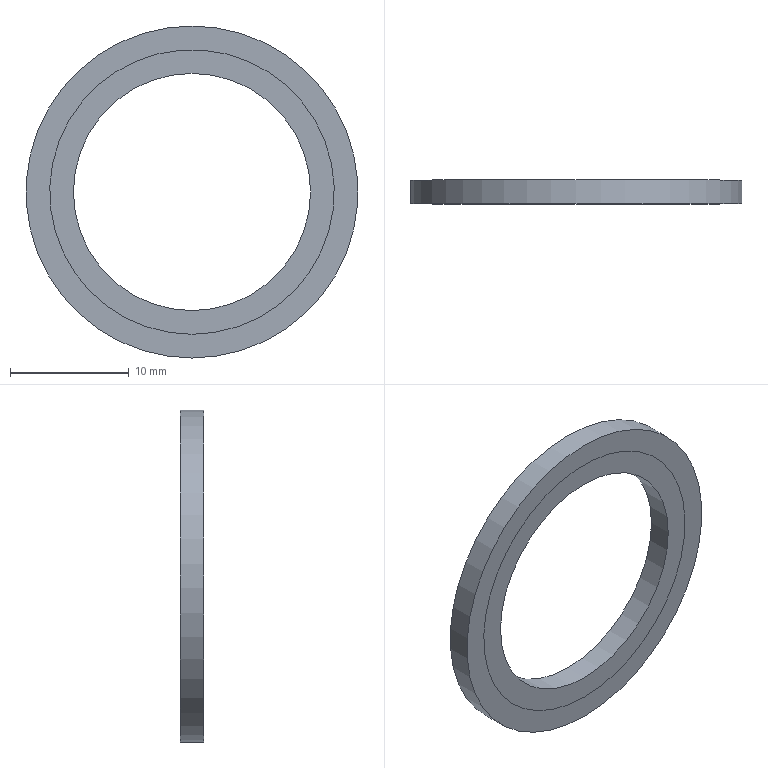Part | STEP file | 8903-ZTZD20 combined gasket | 2 solids | 8 faces | box 28 x 2 x 28 mm | volume 603.186 mm3 | plane 4 | cylinder 4 | commonest cylinder face diameters 24 x2 20 x1 28 x1
STEP:
#1=CARTESIAN_POINT('',(0.,0.,0.));
#2=DIRECTION('',(0.,0.,1.));
#3=DIRECTION('',(1.,0.,0.));
#4=AXIS2_PLACEMENT_3D('',#1,#2,#3);
#5=CARTESIAN_POINT('',(0.,2.,12.));
#6=VERTEX_POINT('',#5);
#7=CARTESIAN_POINT('',(0.,2.,-12.));
#8=VERTEX_POINT('',#7);
#9=CARTESIAN_POINT('',(0.,2.,0.));
#10=DIRECTION('',(0.,1.,0.));
#11=DIRECTION('',(0.,0.,1.));
#12=AXIS2_PLACEMENT_3D('',#9,#10,#11);
#13=CIRCLE('',#12,12.);
#14=CARTESIAN_POINT('',(0.,2.,0.));
#15=DIRECTION('',(0.,1.,0.));
#16=DIRECTION('',(0.,0.,1.));
#17=AXIS2_PLACEMENT_3D('',#14,#15,#16);
#18=PLANE('',#17);
#19=CARTESIAN_POINT('',(0.,0.));
#20=DIRECTION('',(1.,0.));
#21=AXIS2_PLACEMENT_2D('',#19,#20);
#22=CIRCLE('',#21,12.);
#23=(GEOMETRIC_REPRESENTATION_CONTEXT(2)PARAMETRIC_REPRESENTATION_CONTEXT()REPRESENTATION_CONTEXT('',''));
#24=DEFINITIONAL_REPRESENTATION('',(#22),#23);
#25=PCURVE('',#18,#24);
#26=CARTESIAN_POINT('',(0.,-38.212,0.));
#27=DIRECTION('',(0.,-1.,0.));
#28=DIRECTION('',(-1.,0.,0.));
#29=AXIS2_PLACEMENT_3D('',#26,#27,#28);
#30=CYLINDRICAL_SURFACE('',#29,12.);
#31=CARTESIAN_POINT('',(4.712,-40.212));
#32=DIRECTION('',(-1.,0.));
#33=VECTOR('',#32,1.);
#34=LINE('',#31,#33);
#35=(GEOMETRIC_REPRESENTATION_CONTEXT(2)PARAMETRIC_REPRESENTATION_CONTEXT()REPRESENTATION_CONTEXT('',''));
#36=DEFINITIONAL_REPRESENTATION('',(#34),#35);
#37=PCURVE('',#30,#36);
#38=SURFACE_CURVE('',#13,(#25,#37),.PCURVE_S1.);
#39=EDGE_CURVE('',#6,#8,#38,.T.);
#40=ORIENTED_EDGE('',*,*,#39,.F.);
#41=CARTESIAN_POINT('',(0.,2.,0.));
#42=DIRECTION('',(0.,1.,0.));
#43=DIRECTION('',(0.,0.,1.));
#44=AXIS2_PLACEMENT_3D('',#41,#42,#43);
#45=CIRCLE('',#44,12.);
#46=CARTESIAN_POINT('',(0.,0.));
#47=DIRECTION('',(1.,0.));
#48=AXIS2_PLACEMENT_2D('',#46,#47);
#49=CIRCLE('',#48,12.);
#50=(GEOMETRIC_REPRESENTATION_CONTEXT(2)PARAMETRIC_REPRESENTATION_CONTEXT()REPRESENTATION_CONTEXT('',''));
#51=DEFINITIONAL_REPRESENTATION('',(#49),#50);
#52=PCURVE('',#18,#51);
#53=CARTESIAN_POINT('',(10.996,-40.212));
#54=DIRECTION('',(-1.,0.));
#55=VECTOR('',#54,1.);
#56=LINE('',#53,#55);
#57=(GEOMETRIC_REPRESENTATION_CONTEXT(2)PARAMETRIC_REPRESENTATION_CONTEXT()REPRESENTATION_CONTEXT('',''));
#58=DEFINITIONAL_REPRESENTATION('',(#56),#57);
#59=PCURVE('',#30,#58);
#60=SURFACE_CURVE('',#45,(#52,#59),.PCURVE_S1.);
#61=EDGE_CURVE('',#8,#6,#60,.T.);
#62=ORIENTED_EDGE('',*,*,#61,.F.);
#63=EDGE_LOOP('',(#40,#62));
#64=FACE_BOUND('',#63,.T.);
#65=CARTESIAN_POINT('',(0.,2.,14.));
#66=VERTEX_POINT('',#65);
#67=CARTESIAN_POINT('',(0.,2.,-14.));
#68=VERTEX_POINT('',#67);
#69=CARTESIAN_POINT('',(0.,2.,0.));
#70=DIRECTION('',(0.,1.,0.));
#71=DIRECTION('',(0.,0.,1.));
#72=AXIS2_PLACEMENT_3D('',#69,#70,#71);
#73=CIRCLE('',#72,14.);
#74=CARTESIAN_POINT('',(0.,0.));
#75=DIRECTION('',(1.,0.));
#76=AXIS2_PLACEMENT_2D('',#74,#75);
#77=CIRCLE('',#76,14.);
#78=(GEOMETRIC_REPRESENTATION_CONTEXT(2)PARAMETRIC_REPRESENTATION_CONTEXT()REPRESENTATION_CONTEXT('',''));
#79=DEFINITIONAL_REPRESENTATION('',(#77),#78);
#80=PCURVE('',#18,#79);
#81=CARTESIAN_POINT('',(0.,-38.212,0.));
#82=DIRECTION('',(0.,-1.,0.));
#83=DIRECTION('',(-1.,0.,0.));
#84=AXIS2_PLACEMENT_3D('',#81,#82,#83);
#85=CYLINDRICAL_SURFACE('',#84,14.);
#86=CARTESIAN_POINT('',(4.712,-40.212));
#87=DIRECTION('',(-1.,0.));
#88=VECTOR('',#87,1.);
#89=LINE('',#86,#88);
#90=(GEOMETRIC_REPRESENTATION_CONTEXT(2)PARAMETRIC_REPRESENTATION_CONTEXT()REPRESENTATION_CONTEXT('',''));
#91=DEFINITIONAL_REPRESENTATION('',(#89),#90);
#92=PCURVE('',#85,#91);
#93=SURFACE_CURVE('',#73,(#80,#92),.PCURVE_S1.);
#94=EDGE_CURVE('',#66,#68,#93,.T.);
#95=ORIENTED_EDGE('',*,*,#94,.T.);
#96=CARTESIAN_POINT('',(0.,2.,0.));
#97=DIRECTION('',(0.,1.,0.));
#98=DIRECTION('',(0.,0.,1.));
#99=AXIS2_PLACEMENT_3D('',#96,#97,#98);
#100=CIRCLE('',#99,14.);
#101=CARTESIAN_POINT('',(0.,0.));
#102=DIRECTION('',(1.,0.));
#103=AXIS2_PLACEMENT_2D('',#101,#102);
#104=CIRCLE('',#103,14.);
#105=(GEOMETRIC_REPRESENTATION_CONTEXT(2)PARAMETRIC_REPRESENTATION_CONTEXT()REPRESENTATION_CONTEXT('',''));
#106=DEFINITIONAL_REPRESENTATION('',(#104),#105);
#107=PCURVE('',#18,#106);
#108=CARTESIAN_POINT('',(10.996,-40.212));
#109=DIRECTION('',(-1.,0.));
#110=VECTOR('',#109,1.);
#111=LINE('',#108,#110);
#112=(GEOMETRIC_REPRESENTATION_CONTEXT(2)PARAMETRIC_REPRESENTATION_CONTEXT()REPRESENTATION_CONTEXT('',''));
#113=DEFINITIONAL_REPRESENTATION('',(#111),#112);
#114=PCURVE('',#85,#113);
#115=SURFACE_CURVE('',#100,(#107,#114),.PCURVE_S1.);
#116=EDGE_CURVE('',#68,#66,#115,.T.);
#117=ORIENTED_EDGE('',*,*,#116,.T.);
#118=EDGE_LOOP('',(#95,#117));
#119=FACE_BOUND('',#118,.T.);
#120=ADVANCED_FACE('',(#64,#119),#18,.T.);
#121=CARTESIAN_POINT('',(0.,0.,-12.));
#122=VERTEX_POINT('',#121);
#123=CARTESIAN_POINT('',(0.,0.,0.));
#124=DIRECTION('',(0.,-1.,0.));
#125=DIRECTION('',(0.,0.,-1.));
#126=AXIS2_PLACEMENT_3D('',#123,#124,#125);
#127=CIRCLE('',#126,12.);
#128=CARTESIAN_POINT('',(0.,0.,0.));
#129=DIRECTION('',(0.,1.,0.));
#130=DIRECTION('',(0.,0.,1.));
#131=AXIS2_PLACEMENT_3D('',#128,#129,#130);
#132=PLANE('',#131);
#133=CARTESIAN_POINT('',(-12.,0.));
#134=CARTESIAN_POINT('',(-12.,20.785));
#135=CARTESIAN_POINT('',(6.,10.392));
#136=CARTESIAN_POINT('',(24.,0.));
#137=CARTESIAN_POINT('',(6.,-10.392));
#138=CARTESIAN_POINT('',(-12.,-20.785));
#139=CARTESIAN_POINT('',(-12.,0.));
#140=(BOUNDED_CURVE()B_SPLINE_CURVE(2,(#133,#134,#135,#136,#137,#138,#139),.UNSPECIFIED.,.T.,.F.)B_SPLINE_CURVE_WITH_KNOTS((1,2,2,2,2,1),(-2.094,0.,2.094,4.189,6.283,8.378),.UNSPECIFIED.)CURVE()GEOMETRIC_REPRESENTATION_ITEM()RATIONAL_B_SPLINE_CURVE((1.,0.5,1.,0.5,1.,0.5,1.))REPRESENTATION_ITEM(''));
#141=(GEOMETRIC_REPRESENTATION_CONTEXT(2)PARAMETRIC_REPRESENTATION_CONTEXT()REPRESENTATION_CONTEXT('',''));
#142=DEFINITIONAL_REPRESENTATION('',(#140),#141);
#143=PCURVE('',#132,#142);
#144=CARTESIAN_POINT('',(1.571,-38.212));
#145=DIRECTION('',(1.,0.));
#146=VECTOR('',#145,1.);
#147=LINE('',#144,#146);
#148=(GEOMETRIC_REPRESENTATION_CONTEXT(2)PARAMETRIC_REPRESENTATION_CONTEXT()REPRESENTATION_CONTEXT('',''));
#149=DEFINITIONAL_REPRESENTATION('',(#147),#148);
#150=PCURVE('',#30,#149);
#151=SURFACE_CURVE('',#127,(#143,#150),.PCURVE_S1.);
#152=EDGE_CURVE('',#122,#122,#151,.T.);
#153=ORIENTED_EDGE('',*,*,#152,.F.);
#154=EDGE_LOOP('',(#153));
#155=FACE_BOUND('',#154,.T.);
#156=CARTESIAN_POINT('',(0.,0.,-14.));
#157=VERTEX_POINT('',#156);
#158=CARTESIAN_POINT('',(0.,0.,0.));
#159=DIRECTION('',(0.,-1.,0.));
#160=DIRECTION('',(0.,0.,-1.));
#161=AXIS2_PLACEMENT_3D('',#158,#159,#160);
#162=CIRCLE('',#161,14.);
#163=CARTESIAN_POINT('',(-14.,0.));
#164=CARTESIAN_POINT('',(-14.,24.249));
#165=CARTESIAN_POINT('',(7.,12.124));
#166=CARTESIAN_POINT('',(28.,0.));
#167=CARTESIAN_POINT('',(7.,-12.124));
#168=CARTESIAN_POINT('',(-14.,-24.249));
#169=CARTESIAN_POINT('',(-14.,0.));
#170=(BOUNDED_CURVE()B_SPLINE_CURVE(2,(#163,#164,#165,#166,#167,#168,#169),.UNSPECIFIED.,.T.,.F.)B_SPLINE_CURVE_WITH_KNOTS((1,2,2,2,2,1),(-2.094,0.,2.094,4.189,6.283,8.378),.UNSPECIFIED.)CURVE()GEOMETRIC_REPRESENTATION_ITEM()RATIONAL_B_SPLINE_CURVE((1.,0.5,1.,0.5,1.,0.5,1.))REPRESENTATION_ITEM(''));
#171=(GEOMETRIC_REPRESENTATION_CONTEXT(2)PARAMETRIC_REPRESENTATION_CONTEXT()REPRESENTATION_CONTEXT('',''));
#172=DEFINITIONAL_REPRESENTATION('',(#170),#171);
#173=PCURVE('',#132,#172);
#174=CARTESIAN_POINT('',(1.571,-38.212));
#175=DIRECTION('',(1.,0.));
#176=VECTOR('',#175,1.);
#177=LINE('',#174,#176);
#178=(GEOMETRIC_REPRESENTATION_CONTEXT(2)PARAMETRIC_REPRESENTATION_CONTEXT()REPRESENTATION_CONTEXT('',''));
#179=DEFINITIONAL_REPRESENTATION('',(#177),#178);
#180=PCURVE('',#85,#179);
#181=SURFACE_CURVE('',#162,(#173,#180),.PCURVE_S1.);
#182=EDGE_CURVE('',#157,#157,#181,.T.);
#183=ORIENTED_EDGE('',*,*,#182,.T.);
#184=EDGE_LOOP('',(#183));
#185=FACE_BOUND('',#184,.T.);
#186=ADVANCED_FACE('',(#155,#185),#132,.F.);
#187=ORIENTED_EDGE('',*,*,#61,.F.);
#188=CARTESIAN_POINT('',(0.,2.,-12.));
#189=CARTESIAN_POINT('',(0.,0.,-12.));
#190=B_SPLINE_CURVE_WITH_KNOTS('',1,(#188,#189),.UNSPECIFIED.,.F.,.F.,(2,2),(-40.212,-38.212),.PIECEWISE_BEZIER_KNOTS.);
#191=CARTESIAN_POINT('',(7.854,0.));
#192=DIRECTION('',(0.,1.));
#193=VECTOR('',#192,1.);
#194=LINE('',#191,#193);
#195=(GEOMETRIC_REPRESENTATION_CONTEXT(2)PARAMETRIC_REPRESENTATION_CONTEXT()REPRESENTATION_CONTEXT('',''));
#196=DEFINITIONAL_REPRESENTATION('',(#194),#195);
#197=PCURVE('',#30,#196);
#198=CARTESIAN_POINT('',(1.571,0.));
#199=DIRECTION('',(0.,1.));
#200=VECTOR('',#199,1.);
#201=LINE('',#198,#200);
#202=(GEOMETRIC_REPRESENTATION_CONTEXT(2)PARAMETRIC_REPRESENTATION_CONTEXT()REPRESENTATION_CONTEXT('',''));
#203=DEFINITIONAL_REPRESENTATION('',(#201),#202);
#204=PCURVE('',#30,#203);
#205=SEAM_CURVE('',#190,(#197,#204),.PCURVE_S1.);
#206=EDGE_CURVE('',#8,#122,#205,.T.);
#207=ORIENTED_EDGE('',*,*,#206,.T.);
#208=ORIENTED_EDGE('',*,*,#152,.F.);
#209=ORIENTED_EDGE('',*,*,#206,.F.);
#210=ORIENTED_EDGE('',*,*,#39,.F.);
#211=EDGE_LOOP('',(#187,#207,#208,#209,#210));
#212=FACE_BOUND('',#211,.F.);
#213=ADVANCED_FACE('',(#212),#30,.F.);
#214=ORIENTED_EDGE('',*,*,#116,.F.);
#215=CARTESIAN_POINT('',(0.,2.,-14.));
#216=CARTESIAN_POINT('',(0.,0.,-14.));
#217=B_SPLINE_CURVE_WITH_KNOTS('',1,(#215,#216),.UNSPECIFIED.,.F.,.F.,(2,2),(-40.212,-38.212),.PIECEWISE_BEZIER_KNOTS.);
#218=CARTESIAN_POINT('',(7.854,0.));
#219=DIRECTION('',(0.,1.));
#220=VECTOR('',#219,1.);
#221=LINE('',#218,#220);
#222=(GEOMETRIC_REPRESENTATION_CONTEXT(2)PARAMETRIC_REPRESENTATION_CONTEXT()REPRESENTATION_CONTEXT('',''));
#223=DEFINITIONAL_REPRESENTATION('',(#221),#222);
#224=PCURVE('',#85,#223);
#225=CARTESIAN_POINT('',(1.571,0.));
#226=DIRECTION('',(0.,1.));
#227=VECTOR('',#226,1.);
#228=LINE('',#225,#227);
#229=(GEOMETRIC_REPRESENTATION_CONTEXT(2)PARAMETRIC_REPRESENTATION_CONTEXT()REPRESENTATION_CONTEXT('',''));
#230=DEFINITIONAL_REPRESENTATION('',(#228),#229);
#231=PCURVE('',#85,#230);
#232=SEAM_CURVE('',#217,(#224,#231),.PCURVE_S1.);
#233=EDGE_CURVE('',#68,#157,#232,.T.);
#234=ORIENTED_EDGE('',*,*,#233,.T.);
#235=ORIENTED_EDGE('',*,*,#182,.F.);
#236=ORIENTED_EDGE('',*,*,#233,.F.);
#237=ORIENTED_EDGE('',*,*,#94,.F.);
#238=EDGE_LOOP('',(#214,#234,#235,#236,#237));
#239=FACE_BOUND('',#238,.T.);
#240=ADVANCED_FACE('',(#239),#85,.T.);
#241=CLOSED_SHELL('',(#120,#186,#213,#240));
#242=MANIFOLD_SOLID_BREP('',#241);
#243=CARTESIAN_POINT('',(0.,2.,12.));
#244=VERTEX_POINT('',#243);
#245=CARTESIAN_POINT('',(0.,2.,-12.));
#246=VERTEX_POINT('',#245);
#247=CARTESIAN_POINT('',(0.,2.,0.));
#248=DIRECTION('',(0.,1.,0.));
#249=DIRECTION('',(0.,0.,1.));
#250=AXIS2_PLACEMENT_3D('',#247,#248,#249);
#251=CIRCLE('',#250,12.);
#252=CARTESIAN_POINT('',(0.,2.,0.));
#253=DIRECTION('',(0.,1.,0.));
#254=DIRECTION('',(0.,0.,1.));
#255=AXIS2_PLACEMENT_3D('',#252,#253,#254);
#256=PLANE('',#255);
#257=CARTESIAN_POINT('',(0.,0.));
#258=DIRECTION('',(1.,0.));
#259=AXIS2_PLACEMENT_2D('',#257,#258);
#260=CIRCLE('',#259,12.);
#261=(GEOMETRIC_REPRESENTATION_CONTEXT(2)PARAMETRIC_REPRESENTATION_CONTEXT()REPRESENTATION_CONTEXT('',''));
#262=DEFINITIONAL_REPRESENTATION('',(#260),#261);
#263=PCURVE('',#256,#262);
#264=CARTESIAN_POINT('',(0.,-38.212,0.));
#265=DIRECTION('',(0.,-1.,0.));
#266=DIRECTION('',(-1.,0.,0.));
#267=AXIS2_PLACEMENT_3D('',#264,#265,#266);
#268=CYLINDRICAL_SURFACE('',#267,12.);
#269=CARTESIAN_POINT('',(4.712,-40.212));
#270=DIRECTION('',(-1.,0.));
#271=VECTOR('',#270,1.);
#272=LINE('',#269,#271);
#273=(GEOMETRIC_REPRESENTATION_CONTEXT(2)PARAMETRIC_REPRESENTATION_CONTEXT()REPRESENTATION_CONTEXT('',''));
#274=DEFINITIONAL_REPRESENTATION('',(#272),#273);
#275=PCURVE('',#268,#274);
#276=SURFACE_CURVE('',#251,(#263,#275),.PCURVE_S1.);
#277=EDGE_CURVE('',#244,#246,#276,.T.);
#278=ORIENTED_EDGE('',*,*,#277,.T.);
#279=CARTESIAN_POINT('',(0.,2.,0.));
#280=DIRECTION('',(0.,1.,0.));
#281=DIRECTION('',(0.,0.,1.));
#282=AXIS2_PLACEMENT_3D('',#279,#280,#281);
#283=CIRCLE('',#282,12.);
#284=CARTESIAN_POINT('',(0.,0.));
#285=DIRECTION('',(1.,0.));
#286=AXIS2_PLACEMENT_2D('',#284,#285);
#287=CIRCLE('',#286,12.);
#288=(GEOMETRIC_REPRESENTATION_CONTEXT(2)PARAMETRIC_REPRESENTATION_CONTEXT()REPRESENTATION_CONTEXT('',''));
#289=DEFINITIONAL_REPRESENTATION('',(#287),#288);
#290=PCURVE('',#256,#289);
#291=CARTESIAN_POINT('',(10.996,-40.212));
#292=DIRECTION('',(-1.,0.));
#293=VECTOR('',#292,1.);
#294=LINE('',#291,#293);
#295=(GEOMETRIC_REPRESENTATION_CONTEXT(2)PARAMETRIC_REPRESENTATION_CONTEXT()REPRESENTATION_CONTEXT('',''));
#296=DEFINITIONAL_REPRESENTATION('',(#294),#295);
#297=PCURVE('',#268,#296);
#298=SURFACE_CURVE('',#283,(#290,#297),.PCURVE_S1.);
#299=EDGE_CURVE('',#246,#244,#298,.T.);
#300=ORIENTED_EDGE('',*,*,#299,.T.);
#301=EDGE_LOOP('',(#278,#300));
#302=FACE_BOUND('',#301,.T.);
#303=CARTESIAN_POINT('',(0.,2.,10.));
#304=VERTEX_POINT('',#303);
#305=CARTESIAN_POINT('',(0.,2.,-10.));
#306=VERTEX_POINT('',#305);
#307=CARTESIAN_POINT('',(0.,2.,0.));
#308=DIRECTION('',(0.,1.,0.));
#309=DIRECTION('',(0.,0.,1.));
#310=AXIS2_PLACEMENT_3D('',#307,#308,#309);
#311=CIRCLE('',#310,10.);
#312=CARTESIAN_POINT('',(0.,0.));
#313=DIRECTION('',(1.,0.));
#314=AXIS2_PLACEMENT_2D('',#312,#313);
#315=CIRCLE('',#314,10.);
#316=(GEOMETRIC_REPRESENTATION_CONTEXT(2)PARAMETRIC_REPRESENTATION_CONTEXT()REPRESENTATION_CONTEXT('',''));
#317=DEFINITIONAL_REPRESENTATION('',(#315),#316);
#318=PCURVE('',#256,#317);
#319=CARTESIAN_POINT('',(0.,-38.212,0.));
#320=DIRECTION('',(0.,-1.,0.));
#321=DIRECTION('',(-1.,0.,0.));
#322=AXIS2_PLACEMENT_3D('',#319,#320,#321);
#323=CYLINDRICAL_SURFACE('',#322,10.);
#324=CARTESIAN_POINT('',(4.712,-40.212));
#325=DIRECTION('',(-1.,0.));
#326=VECTOR('',#325,1.);
#327=LINE('',#324,#326);
#328=(GEOMETRIC_REPRESENTATION_CONTEXT(2)PARAMETRIC_REPRESENTATION_CONTEXT()REPRESENTATION_CONTEXT('',''));
#329=DEFINITIONAL_REPRESENTATION('',(#327),#328);
#330=PCURVE('',#323,#329);
#331=SURFACE_CURVE('',#311,(#318,#330),.PCURVE_S1.);
#332=EDGE_CURVE('',#304,#306,#331,.T.);
#333=ORIENTED_EDGE('',*,*,#332,.F.);
#334=CARTESIAN_POINT('',(0.,2.,0.));
#335=DIRECTION('',(0.,1.,0.));
#336=DIRECTION('',(0.,0.,1.));
#337=AXIS2_PLACEMENT_3D('',#334,#335,#336);
#338=CIRCLE('',#337,10.);
#339=CARTESIAN_POINT('',(0.,0.));
#340=DIRECTION('',(1.,0.));
#341=AXIS2_PLACEMENT_2D('',#339,#340);
#342=CIRCLE('',#341,10.);
#343=(GEOMETRIC_REPRESENTATION_CONTEXT(2)PARAMETRIC_REPRESENTATION_CONTEXT()REPRESENTATION_CONTEXT('',''));
#344=DEFINITIONAL_REPRESENTATION('',(#342),#343);
#345=PCURVE('',#256,#344);
#346=CARTESIAN_POINT('',(10.996,-40.212));
#347=DIRECTION('',(-1.,0.));
#348=VECTOR('',#347,1.);
#349=LINE('',#346,#348);
#350=(GEOMETRIC_REPRESENTATION_CONTEXT(2)PARAMETRIC_REPRESENTATION_CONTEXT()REPRESENTATION_CONTEXT('',''));
#351=DEFINITIONAL_REPRESENTATION('',(#349),#350);
#352=PCURVE('',#323,#351);
#353=SURFACE_CURVE('',#338,(#345,#352),.PCURVE_S1.);
#354=EDGE_CURVE('',#306,#304,#353,.T.);
#355=ORIENTED_EDGE('',*,*,#354,.F.);
#356=EDGE_LOOP('',(#333,#355));
#357=FACE_BOUND('',#356,.T.);
#358=ADVANCED_FACE('',(#302,#357),#256,.T.);
#359=CARTESIAN_POINT('',(0.,0.,-12.));
#360=VERTEX_POINT('',#359);
#361=CARTESIAN_POINT('',(0.,0.,0.));
#362=DIRECTION('',(0.,-1.,0.));
#363=DIRECTION('',(0.,0.,-1.));
#364=AXIS2_PLACEMENT_3D('',#361,#362,#363);
#365=CIRCLE('',#364,12.);
#366=CARTESIAN_POINT('',(0.,0.,0.));
#367=DIRECTION('',(0.,1.,0.));
#368=DIRECTION('',(0.,0.,1.));
#369=AXIS2_PLACEMENT_3D('',#366,#367,#368);
#370=PLANE('',#369);
#371=CARTESIAN_POINT('',(-12.,0.));
#372=CARTESIAN_POINT('',(-12.,20.785));
#373=CARTESIAN_POINT('',(6.,10.392));
#374=CARTESIAN_POINT('',(24.,0.));
#375=CARTESIAN_POINT('',(6.,-10.392));
#376=CARTESIAN_POINT('',(-12.,-20.785));
#377=CARTESIAN_POINT('',(-12.,0.));
#378=(BOUNDED_CURVE()B_SPLINE_CURVE(2,(#371,#372,#373,#374,#375,#376,#377),.UNSPECIFIED.,.T.,.F.)B_SPLINE_CURVE_WITH_KNOTS((1,2,2,2,2,1),(-2.094,0.,2.094,4.189,6.283,8.378),.UNSPECIFIED.)CURVE()GEOMETRIC_REPRESENTATION_ITEM()RATIONAL_B_SPLINE_CURVE((1.,0.5,1.,0.5,1.,0.5,1.))REPRESENTATION_ITEM(''));
#379=(GEOMETRIC_REPRESENTATION_CONTEXT(2)PARAMETRIC_REPRESENTATION_CONTEXT()REPRESENTATION_CONTEXT('',''));
#380=DEFINITIONAL_REPRESENTATION('',(#378),#379);
#381=PCURVE('',#370,#380);
#382=CARTESIAN_POINT('',(1.571,-38.212));
#383=DIRECTION('',(1.,0.));
#384=VECTOR('',#383,1.);
#385=LINE('',#382,#384);
#386=(GEOMETRIC_REPRESENTATION_CONTEXT(2)PARAMETRIC_REPRESENTATION_CONTEXT()REPRESENTATION_CONTEXT('',''));
#387=DEFINITIONAL_REPRESENTATION('',(#385),#386);
#388=PCURVE('',#268,#387);
#389=SURFACE_CURVE('',#365,(#381,#388),.PCURVE_S1.);
#390=EDGE_CURVE('',#360,#360,#389,.T.);
#391=ORIENTED_EDGE('',*,*,#390,.T.);
#392=EDGE_LOOP('',(#391));
#393=FACE_BOUND('',#392,.T.);
#394=CARTESIAN_POINT('',(0.,0.,-10.));
#395=VERTEX_POINT('',#394);
#396=CARTESIAN_POINT('',(0.,0.,0.));
#397=DIRECTION('',(0.,-1.,0.));
#398=DIRECTION('',(0.,0.,-1.));
#399=AXIS2_PLACEMENT_3D('',#396,#397,#398);
#400=CIRCLE('',#399,10.);
#401=CARTESIAN_POINT('',(-10.,0.));
#402=CARTESIAN_POINT('',(-10.,17.321));
#403=CARTESIAN_POINT('',(5.,8.66));
#404=CARTESIAN_POINT('',(20.,0.));
#405=CARTESIAN_POINT('',(5.,-8.66));
#406=CARTESIAN_POINT('',(-10.,-17.321));
#407=CARTESIAN_POINT('',(-10.,0.));
#408=(BOUNDED_CURVE()B_SPLINE_CURVE(2,(#401,#402,#403,#404,#405,#406,#407),.UNSPECIFIED.,.T.,.F.)B_SPLINE_CURVE_WITH_KNOTS((1,2,2,2,2,1),(-2.094,0.,2.094,4.189,6.283,8.378),.UNSPECIFIED.)CURVE()GEOMETRIC_REPRESENTATION_ITEM()RATIONAL_B_SPLINE_CURVE((1.,0.5,1.,0.5,1.,0.5,1.))REPRESENTATION_ITEM(''));
#409=(GEOMETRIC_REPRESENTATION_CONTEXT(2)PARAMETRIC_REPRESENTATION_CONTEXT()REPRESENTATION_CONTEXT('',''));
#410=DEFINITIONAL_REPRESENTATION('',(#408),#409);
#411=PCURVE('',#370,#410);
#412=CARTESIAN_POINT('',(1.571,-38.212));
#413=DIRECTION('',(1.,0.));
#414=VECTOR('',#413,1.);
#415=LINE('',#412,#414);
#416=(GEOMETRIC_REPRESENTATION_CONTEXT(2)PARAMETRIC_REPRESENTATION_CONTEXT()REPRESENTATION_CONTEXT('',''));
#417=DEFINITIONAL_REPRESENTATION('',(#415),#416);
#418=PCURVE('',#323,#417);
#419=SURFACE_CURVE('',#400,(#411,#418),.PCURVE_S1.);
#420=EDGE_CURVE('',#395,#395,#419,.T.);
#421=ORIENTED_EDGE('',*,*,#420,.F.);
#422=EDGE_LOOP('',(#421));
#423=FACE_BOUND('',#422,.T.);
#424=ADVANCED_FACE('',(#393,#423),#370,.F.);
#425=ORIENTED_EDGE('',*,*,#299,.F.);
#426=CARTESIAN_POINT('',(0.,2.,-12.));
#427=CARTESIAN_POINT('',(0.,0.,-12.));
#428=B_SPLINE_CURVE_WITH_KNOTS('',1,(#426,#427),.UNSPECIFIED.,.F.,.F.,(2,2),(-40.212,-38.212),.PIECEWISE_BEZIER_KNOTS.);
#429=CARTESIAN_POINT('',(7.854,0.));
#430=DIRECTION('',(0.,1.));
#431=VECTOR('',#430,1.);
#432=LINE('',#429,#431);
#433=(GEOMETRIC_REPRESENTATION_CONTEXT(2)PARAMETRIC_REPRESENTATION_CONTEXT()REPRESENTATION_CONTEXT('',''));
#434=DEFINITIONAL_REPRESENTATION('',(#432),#433);
#435=PCURVE('',#268,#434);
#436=CARTESIAN_POINT('',(1.571,0.));
#437=DIRECTION('',(0.,1.));
#438=VECTOR('',#437,1.);
#439=LINE('',#436,#438);
#440=(GEOMETRIC_REPRESENTATION_CONTEXT(2)PARAMETRIC_REPRESENTATION_CONTEXT()REPRESENTATION_CONTEXT('',''));
#441=DEFINITIONAL_REPRESENTATION('',(#439),#440);
#442=PCURVE('',#268,#441);
#443=SEAM_CURVE('',#428,(#435,#442),.PCURVE_S1.);
#444=EDGE_CURVE('',#246,#360,#443,.T.);
#445=ORIENTED_EDGE('',*,*,#444,.T.);
#446=ORIENTED_EDGE('',*,*,#390,.F.);
#447=ORIENTED_EDGE('',*,*,#444,.F.);
#448=ORIENTED_EDGE('',*,*,#277,.F.);
#449=EDGE_LOOP('',(#425,#445,#446,#447,#448));
#450=FACE_BOUND('',#449,.T.);
#451=ADVANCED_FACE('',(#450),#268,.T.);
#452=ORIENTED_EDGE('',*,*,#354,.F.);
#453=CARTESIAN_POINT('',(0.,2.,-10.));
#454=CARTESIAN_POINT('',(0.,0.,-10.));
#455=B_SPLINE_CURVE_WITH_KNOTS('',1,(#453,#454),.UNSPECIFIED.,.F.,.F.,(2,2),(-40.212,-38.212),.PIECEWISE_BEZIER_KNOTS.);
#456=CARTESIAN_POINT('',(7.854,0.));
#457=DIRECTION('',(0.,1.));
#458=VECTOR('',#457,1.);
#459=LINE('',#456,#458);
#460=(GEOMETRIC_REPRESENTATION_CONTEXT(2)PARAMETRIC_REPRESENTATION_CONTEXT()REPRESENTATION_CONTEXT('',''));
#461=DEFINITIONAL_REPRESENTATION('',(#459),#460);
#462=PCURVE('',#323,#461);
#463=CARTESIAN_POINT('',(1.571,0.));
#464=DIRECTION('',(0.,1.));
#465=VECTOR('',#464,1.);
#466=LINE('',#463,#465);
#467=(GEOMETRIC_REPRESENTATION_CONTEXT(2)PARAMETRIC_REPRESENTATION_CONTEXT()REPRESENTATION_CONTEXT('',''));
#468=DEFINITIONAL_REPRESENTATION('',(#466),#467);
#469=PCURVE('',#323,#468);
#470=SEAM_CURVE('',#455,(#462,#469),.PCURVE_S1.);
#471=EDGE_CURVE('',#306,#395,#470,.T.);
#472=ORIENTED_EDGE('',*,*,#471,.T.);
#473=ORIENTED_EDGE('',*,*,#420,.F.);
#474=ORIENTED_EDGE('',*,*,#471,.F.);
#475=ORIENTED_EDGE('',*,*,#332,.F.);
#476=EDGE_LOOP('',(#452,#472,#473,#474,#475));
#477=FACE_BOUND('',#476,.F.);
#478=ADVANCED_FACE('',(#477),#323,.F.);
#479=CLOSED_SHELL('',(#358,#424,#451,#478));
#480=MANIFOLD_SOLID_BREP('',#479);
#481=(LENGTH_UNIT()NAMED_UNIT(*)SI_UNIT(.MILLI.,.METRE.));
#482=UNCERTAINTY_MEASURE_WITH_UNIT(LENGTH_MEASURE(0.000005),#481,'','');
#483=(NAMED_UNIT(*)PLANE_ANGLE_UNIT()SI_UNIT($,.RADIAN.));
#484=(NAMED_UNIT(*)SI_UNIT($,.STERADIAN.)SOLID_ANGLE_UNIT());
#485=(GEOMETRIC_REPRESENTATION_CONTEXT(3)GLOBAL_UNCERTAINTY_ASSIGNED_CONTEXT((#482))GLOBAL_UNIT_ASSIGNED_CONTEXT((#481,#483,#484))REPRESENTATION_CONTEXT('',''));
#486=SHAPE_REPRESENTATION('',(#4,#242,#480),#485);